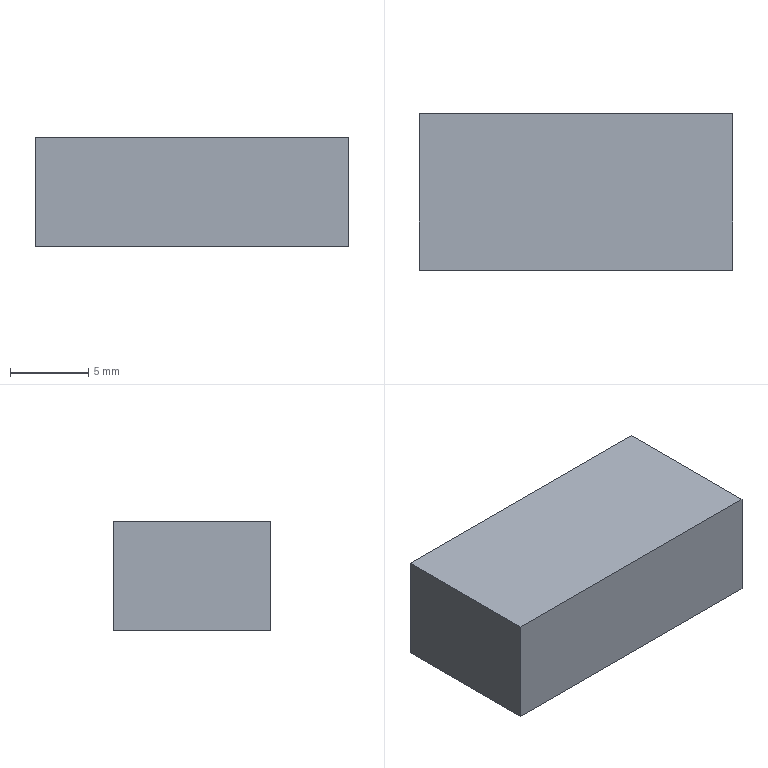Part | SolidWorks | features Extrusion 1 | 1 solid | 6 faces | box 20 x 10 x 7 mm | volume 1400 mm3 | plane 6
STEP:
#1=CARTESIAN_POINT('',(-10.,5.,3.5));
#2=VERTEX_POINT('',#1);
#3=CARTESIAN_POINT('',(-10.,-5.,3.5));
#4=VERTEX_POINT('',#3);
#5=CARTESIAN_POINT('',(-10.,5.,3.5));
#6=DIRECTION('',(0.,-1.,0.));
#7=VECTOR('',#6,1000.);
#8=LINE('',#5,#7);
#9=EDGE_CURVE('',#2,#4,#8,.T.);
#10=ORIENTED_EDGE('',*,*,#9,.F.);
#11=CARTESIAN_POINT('',(-10.,5.,-3.5));
#12=VERTEX_POINT('',#11);
#13=CARTESIAN_POINT('',(-10.,5.,-3.5));
#14=DIRECTION('',(0.,0.,1.));
#15=VECTOR('',#14,1000.);
#16=LINE('',#13,#15);
#17=EDGE_CURVE('',#12,#2,#16,.T.);
#18=ORIENTED_EDGE('',*,*,#17,.F.);
#19=CARTESIAN_POINT('',(-10.,-5.,-3.5));
#20=VERTEX_POINT('',#19);
#21=CARTESIAN_POINT('',(-10.,5.,-3.5));
#22=DIRECTION('',(0.,-1.,0.));
#23=VECTOR('',#22,1000.);
#24=LINE('',#21,#23);
#25=EDGE_CURVE('',#12,#20,#24,.T.);
#26=ORIENTED_EDGE('',*,*,#25,.T.);
#27=CARTESIAN_POINT('',(-10.,-5.,-3.5));
#28=DIRECTION('',(0.,0.,1.));
#29=VECTOR('',#28,1000.);
#30=LINE('',#27,#29);
#31=EDGE_CURVE('',#20,#4,#30,.T.);
#32=ORIENTED_EDGE('',*,*,#31,.T.);
#33=EDGE_LOOP('',(#10,#18,#26,#32));
#34=FACE_OUTER_BOUND('',#33,.T.);
#35=CARTESIAN_POINT('',(-10.,5.,-3.5));
#36=DIRECTION('',(-1.,0.,0.));
#37=DIRECTION('',(0.,0.,1.));
#38=AXIS2_PLACEMENT_3D('',#35,#36,#37);
#39=PLANE('',#38);
#40=ADVANCED_FACE('',(#34),#39,.T.);
#41=CARTESIAN_POINT('',(10.,5.,3.5));
#42=VERTEX_POINT('',#41);
#43=CARTESIAN_POINT('',(10.,5.,3.5));
#44=DIRECTION('',(-1.,0.,0.));
#45=VECTOR('',#44,1000.);
#46=LINE('',#43,#45);
#47=EDGE_CURVE('',#42,#2,#46,.T.);
#48=ORIENTED_EDGE('',*,*,#47,.F.);
#49=CARTESIAN_POINT('',(10.,5.,-3.5));
#50=VERTEX_POINT('',#49);
#51=CARTESIAN_POINT('',(10.,5.,-3.5));
#52=DIRECTION('',(0.,0.,1.));
#53=VECTOR('',#52,1000.);
#54=LINE('',#51,#53);
#55=EDGE_CURVE('',#50,#42,#54,.T.);
#56=ORIENTED_EDGE('',*,*,#55,.F.);
#57=CARTESIAN_POINT('',(10.,5.,-3.5));
#58=DIRECTION('',(-1.,0.,0.));
#59=VECTOR('',#58,1000.);
#60=LINE('',#57,#59);
#61=EDGE_CURVE('',#50,#12,#60,.T.);
#62=ORIENTED_EDGE('',*,*,#61,.T.);
#63=ORIENTED_EDGE('',*,*,#17,.T.);
#64=EDGE_LOOP('',(#48,#56,#62,#63));
#65=FACE_OUTER_BOUND('',#64,.T.);
#66=CARTESIAN_POINT('',(10.,5.,-3.5));
#67=DIRECTION('',(0.,1.,0.));
#68=DIRECTION('',(0.,0.,1.));
#69=AXIS2_PLACEMENT_3D('',#66,#67,#68);
#70=PLANE('',#69);
#71=ADVANCED_FACE('',(#65),#70,.T.);
#72=CARTESIAN_POINT('',(10.,-5.,3.5));
#73=VERTEX_POINT('',#72);
#74=CARTESIAN_POINT('',(10.,-5.,3.5));
#75=DIRECTION('',(0.,1.,0.));
#76=VECTOR('',#75,1000.);
#77=LINE('',#74,#76);
#78=EDGE_CURVE('',#73,#42,#77,.T.);
#79=ORIENTED_EDGE('',*,*,#78,.F.);
#80=CARTESIAN_POINT('',(10.,-5.,-3.5));
#81=VERTEX_POINT('',#80);
#82=CARTESIAN_POINT('',(10.,-5.,-3.5));
#83=DIRECTION('',(0.,0.,1.));
#84=VECTOR('',#83,1000.);
#85=LINE('',#82,#84);
#86=EDGE_CURVE('',#81,#73,#85,.T.);
#87=ORIENTED_EDGE('',*,*,#86,.F.);
#88=CARTESIAN_POINT('',(10.,-5.,-3.5));
#89=DIRECTION('',(0.,1.,0.));
#90=VECTOR('',#89,1000.);
#91=LINE('',#88,#90);
#92=EDGE_CURVE('',#81,#50,#91,.T.);
#93=ORIENTED_EDGE('',*,*,#92,.T.);
#94=ORIENTED_EDGE('',*,*,#55,.T.);
#95=EDGE_LOOP('',(#79,#87,#93,#94));
#96=FACE_OUTER_BOUND('',#95,.T.);
#97=CARTESIAN_POINT('',(10.,-5.,-3.5));
#98=DIRECTION('',(1.,0.,0.));
#99=DIRECTION('',(0.,0.,-1.));
#100=AXIS2_PLACEMENT_3D('',#97,#98,#99);
#101=PLANE('',#100);
#102=ADVANCED_FACE('',(#96),#101,.T.);
#103=CARTESIAN_POINT('',(-10.,-5.,3.5));
#104=DIRECTION('',(1.,0.,0.));
#105=VECTOR('',#104,1000.);
#106=LINE('',#103,#105);
#107=EDGE_CURVE('',#4,#73,#106,.T.);
#108=ORIENTED_EDGE('',*,*,#107,.F.);
#109=ORIENTED_EDGE('',*,*,#31,.F.);
#110=CARTESIAN_POINT('',(-10.,-5.,-3.5));
#111=DIRECTION('',(1.,0.,0.));
#112=VECTOR('',#111,1000.);
#113=LINE('',#110,#112);
#114=EDGE_CURVE('',#20,#81,#113,.T.);
#115=ORIENTED_EDGE('',*,*,#114,.T.);
#116=ORIENTED_EDGE('',*,*,#86,.T.);
#117=EDGE_LOOP('',(#108,#109,#115,#116));
#118=FACE_OUTER_BOUND('',#117,.T.);
#119=CARTESIAN_POINT('',(-10.,-5.,-3.5));
#120=DIRECTION('',(0.,-1.,0.));
#121=DIRECTION('',(0.,0.,-1.));
#122=AXIS2_PLACEMENT_3D('',#119,#120,#121);
#123=PLANE('',#122);
#124=ADVANCED_FACE('',(#118),#123,.T.);
#125=ORIENTED_EDGE('',*,*,#25,.F.);
#126=ORIENTED_EDGE('',*,*,#61,.F.);
#127=ORIENTED_EDGE('',*,*,#92,.F.);
#128=ORIENTED_EDGE('',*,*,#114,.F.);
#129=EDGE_LOOP('',(#125,#126,#127,#128));
#130=FACE_OUTER_BOUND('',#129,.T.);
#131=CARTESIAN_POINT('',(0.,0.,-3.5));
#132=DIRECTION('',(0.,0.,1.));
#133=DIRECTION('',(1.,0.,0.));
#134=AXIS2_PLACEMENT_3D('',#131,#132,#133);
#135=PLANE('',#134);
#136=ADVANCED_FACE('',(#130),#135,.F.);
#137=ORIENTED_EDGE('',*,*,#9,.T.);
#138=ORIENTED_EDGE('',*,*,#107,.T.);
#139=ORIENTED_EDGE('',*,*,#78,.T.);
#140=ORIENTED_EDGE('',*,*,#47,.T.);
#141=EDGE_LOOP('',(#137,#138,#139,#140));
#142=FACE_OUTER_BOUND('',#141,.T.);
#143=CARTESIAN_POINT('',(0.,0.,3.5));
#144=DIRECTION('',(0.,0.,1.));
#145=DIRECTION('',(1.,0.,0.));
#146=AXIS2_PLACEMENT_3D('',#143,#144,#145);
#147=PLANE('',#146);
#148=ADVANCED_FACE('',(#142),#147,.T.);
#149=CLOSED_SHELL('',(#40,#71,#102,#124,#136,#148));
#150=MANIFOLD_SOLID_BREP('',#149);
#151=CARTESIAN_POINT('',(0.,0.,0.));
#152=DIRECTION('',(0.,0.,1.));
#153=DIRECTION('',(1.,0.,0.));
#154=AXIS2_PLACEMENT_3D('',#151,#152,#153);
#155=(LENGTH_UNIT()NAMED_UNIT(*)SI_UNIT(.MILLI.,.METRE.));
#156=UNCERTAINTY_MEASURE_WITH_UNIT(LENGTH_MEASURE(0.00001),#155,'','');
#157=(NAMED_UNIT(*)PLANE_ANGLE_UNIT()SI_UNIT($,.RADIAN.));
#158=(NAMED_UNIT(*)SI_UNIT($,.STERADIAN.)SOLID_ANGLE_UNIT());
#159=(GEOMETRIC_REPRESENTATION_CONTEXT(3)GLOBAL_UNCERTAINTY_ASSIGNED_CONTEXT((#156))GLOBAL_UNIT_ASSIGNED_CONTEXT((#155,#157,#158))REPRESENTATION_CONTEXT('',''));
#160=ADVANCED_BREP_SHAPE_REPRESENTATION('',(#150,#154),#159);